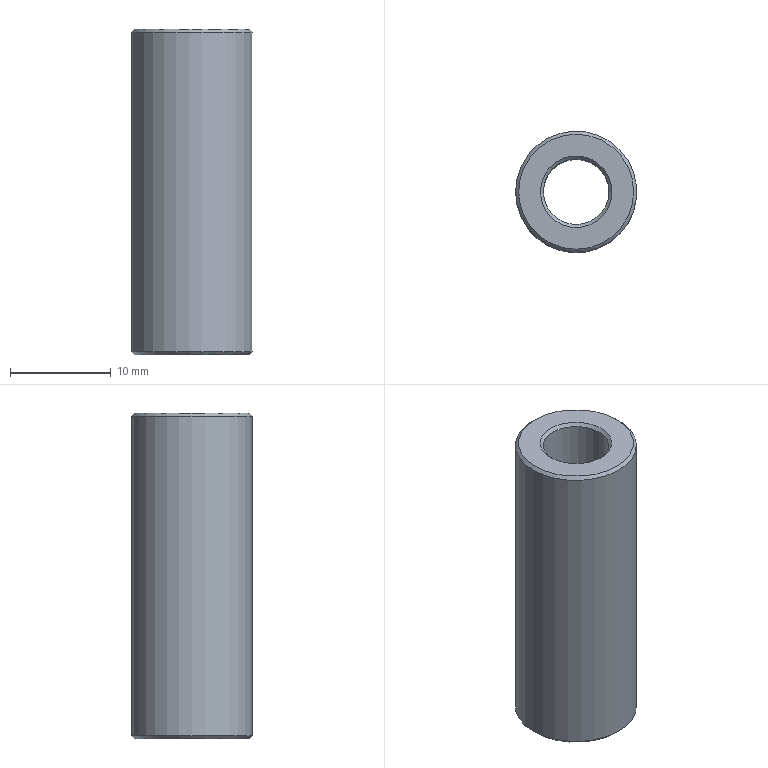Part | STEP file | 200 mesh_id1326 | 1 solid | 8 faces | box 12 x 12 x 32.3 mm | volume 2576 mm3 | cone 4 | plane 2 | cylinder 2 | commonest cylinder face diameters 6.5 x1 12 x1
STEP:
#1=CARTESIAN_POINT('',(-16971.698,-4073.269,32.1));
#2=VERTEX_POINT('',#1);
#3=CARTESIAN_POINT('',(-16968.148,-4073.269,32.1));
#4=DIRECTION('',(0.,0.,-1.));
#5=DIRECTION('',(-1.,0.,0.));
#6=AXIS2_PLACEMENT_3D('',#3,#4,#5);
#7=CIRCLE('',#6,3.55);
#8=EDGE_CURVE('',#2,#2,#7,.T.);
#9=ORIENTED_EDGE('',*,*,#8,.T.);
#10=EDGE_LOOP('',(#9));
#11=FACE_BOUND('',#10,.T.);
#12=CARTESIAN_POINT('',(-16973.848,-4073.269,32.1));
#13=VERTEX_POINT('',#12);
#14=CARTESIAN_POINT('',(-16968.148,-4073.269,32.1));
#15=DIRECTION('',(0.,0.,1.));
#16=DIRECTION('',(-1.,0.,0.));
#17=AXIS2_PLACEMENT_3D('',#14,#15,#16);
#18=CIRCLE('',#17,5.7);
#19=EDGE_CURVE('',#13,#13,#18,.T.);
#20=ORIENTED_EDGE('',*,*,#19,.T.);
#21=EDGE_LOOP('',(#20));
#22=FACE_BOUND('',#21,.T.);
#23=CARTESIAN_POINT('',(-16968.148,-4073.269,32.1));
#24=DIRECTION('',(0.,0.,1.));
#25=DIRECTION('',(-1.,0.,0.));
#26=AXIS2_PLACEMENT_3D('',#23,#24,#25);
#27=PLANE('',#26);
#28=ADVANCED_FACE('',(#11,#22),#27,.T.);
#29=CARTESIAN_POINT('',(-16974.148,-4073.269,0.1));
#30=VERTEX_POINT('',#29);
#31=CARTESIAN_POINT('',(-16968.148,-4073.269,0.1));
#32=DIRECTION('',(0.,0.,1.));
#33=DIRECTION('',(-1.,0.,0.));
#34=AXIS2_PLACEMENT_3D('',#31,#32,#33);
#35=CIRCLE('',#34,6.);
#36=EDGE_CURVE('',#30,#30,#35,.T.);
#37=ORIENTED_EDGE('',*,*,#36,.T.);
#38=EDGE_LOOP('',(#37));
#39=FACE_BOUND('',#38,.T.);
#40=CARTESIAN_POINT('',(-16974.148,-4073.269,31.8));
#41=VERTEX_POINT('',#40);
#42=CARTESIAN_POINT('',(-16968.148,-4073.269,31.8));
#43=DIRECTION('',(0.,0.,-1.));
#44=DIRECTION('',(-1.,0.,0.));
#45=AXIS2_PLACEMENT_3D('',#42,#43,#44);
#46=CIRCLE('',#45,6.);
#47=EDGE_CURVE('',#41,#41,#46,.T.);
#48=ORIENTED_EDGE('',*,*,#47,.T.);
#49=EDGE_LOOP('',(#48));
#50=FACE_BOUND('',#49,.T.);
#51=CARTESIAN_POINT('',(-16968.148,-4073.269,32.4));
#52=DIRECTION('',(0.,0.,-1.));
#53=DIRECTION('',(-1.,0.,0.));
#54=AXIS2_PLACEMENT_3D('',#51,#52,#53);
#55=CYLINDRICAL_SURFACE('',#54,6.);
#56=ADVANCED_FACE('',(#39,#50),#55,.T.);
#57=CARTESIAN_POINT('',(-16971.698,-4073.269,-0.2));
#58=VERTEX_POINT('',#57);
#59=CARTESIAN_POINT('',(-16968.148,-4073.269,-0.2));
#60=DIRECTION('',(0.,0.,1.));
#61=DIRECTION('',(-1.,0.,0.));
#62=AXIS2_PLACEMENT_3D('',#59,#60,#61);
#63=CIRCLE('',#62,3.55);
#64=EDGE_CURVE('',#58,#58,#63,.T.);
#65=ORIENTED_EDGE('',*,*,#64,.T.);
#66=EDGE_LOOP('',(#65));
#67=FACE_BOUND('',#66,.T.);
#68=CARTESIAN_POINT('',(-16973.848,-4073.269,-0.2));
#69=VERTEX_POINT('',#68);
#70=CARTESIAN_POINT('',(-16968.148,-4073.269,-0.2));
#71=DIRECTION('',(0.,0.,-1.));
#72=DIRECTION('',(-1.,0.,0.));
#73=AXIS2_PLACEMENT_3D('',#70,#71,#72);
#74=CIRCLE('',#73,5.7);
#75=EDGE_CURVE('',#69,#69,#74,.T.);
#76=ORIENTED_EDGE('',*,*,#75,.T.);
#77=EDGE_LOOP('',(#76));
#78=FACE_BOUND('',#77,.T.);
#79=CARTESIAN_POINT('',(-16968.148,-4073.269,-0.2));
#80=DIRECTION('',(0.,0.,1.));
#81=DIRECTION('',(-1.,0.,0.));
#82=AXIS2_PLACEMENT_3D('',#79,#80,#81);
#83=PLANE('',#82);
#84=ADVANCED_FACE('',(#67,#78),#83,.F.);
#85=CARTESIAN_POINT('',(-16971.398,-4073.269,0.1));
#86=VERTEX_POINT('',#85);
#87=CARTESIAN_POINT('',(-16968.148,-4073.269,0.1));
#88=DIRECTION('',(0.,0.,-1.));
#89=DIRECTION('',(-1.,0.,0.));
#90=AXIS2_PLACEMENT_3D('',#87,#88,#89);
#91=CIRCLE('',#90,3.25);
#92=EDGE_CURVE('',#86,#86,#91,.T.);
#93=ORIENTED_EDGE('',*,*,#92,.T.);
#94=EDGE_LOOP('',(#93));
#95=FACE_BOUND('',#94,.T.);
#96=CARTESIAN_POINT('',(-16971.398,-4073.269,31.8));
#97=VERTEX_POINT('',#96);
#98=CARTESIAN_POINT('',(-16968.148,-4073.269,31.8));
#99=DIRECTION('',(0.,0.,1.));
#100=DIRECTION('',(-1.,0.,0.));
#101=AXIS2_PLACEMENT_3D('',#98,#99,#100);
#102=CIRCLE('',#101,3.25);
#103=EDGE_CURVE('',#97,#97,#102,.T.);
#104=ORIENTED_EDGE('',*,*,#103,.T.);
#105=EDGE_LOOP('',(#104));
#106=FACE_BOUND('',#105,.T.);
#107=CARTESIAN_POINT('',(-16968.148,-4073.269,32.4));
#108=DIRECTION('',(0.,0.,-1.));
#109=DIRECTION('',(1.,0.,0.));
#110=AXIS2_PLACEMENT_3D('',#107,#108,#109);
#111=CYLINDRICAL_SURFACE('',#110,3.25);
#112=ADVANCED_FACE('',(#95,#106),#111,.F.);
#113=ORIENTED_EDGE('',*,*,#103,.F.);
#114=EDGE_LOOP('',(#113));
#115=FACE_BOUND('',#114,.T.);
#116=ORIENTED_EDGE('',*,*,#8,.F.);
#117=EDGE_LOOP('',(#116));
#118=FACE_BOUND('',#117,.T.);
#119=CARTESIAN_POINT('',(-16968.148,-4073.269,32.1));
#120=DIRECTION('',(0.,0.,1.));
#121=DIRECTION('',(-1.,0.,0.));
#122=AXIS2_PLACEMENT_3D('',#119,#120,#121);
#123=CONICAL_SURFACE('',#122,3.55,45.);
#124=ADVANCED_FACE('',(#115,#118),#123,.F.);
#125=ORIENTED_EDGE('',*,*,#19,.F.);
#126=EDGE_LOOP('',(#125));
#127=FACE_BOUND('',#126,.T.);
#128=ORIENTED_EDGE('',*,*,#47,.F.);
#129=EDGE_LOOP('',(#128));
#130=FACE_BOUND('',#129,.T.);
#131=CARTESIAN_POINT('',(-16968.148,-4073.269,31.8));
#132=DIRECTION('',(0.,0.,-1.));
#133=DIRECTION('',(1.,0.,0.));
#134=AXIS2_PLACEMENT_3D('',#131,#132,#133);
#135=CONICAL_SURFACE('',#134,6.,45.);
#136=ADVANCED_FACE('',(#127,#130),#135,.T.);
#137=ORIENTED_EDGE('',*,*,#92,.F.);
#138=EDGE_LOOP('',(#137));
#139=FACE_BOUND('',#138,.T.);
#140=ORIENTED_EDGE('',*,*,#64,.F.);
#141=EDGE_LOOP('',(#140));
#142=FACE_BOUND('',#141,.T.);
#143=CARTESIAN_POINT('',(-16968.148,-4073.269,-0.2));
#144=DIRECTION('',(0.,0.,-1.));
#145=DIRECTION('',(1.,0.,0.));
#146=AXIS2_PLACEMENT_3D('',#143,#144,#145);
#147=CONICAL_SURFACE('',#146,3.55,45.);
#148=ADVANCED_FACE('',(#139,#142),#147,.F.);
#149=ORIENTED_EDGE('',*,*,#75,.F.);
#150=EDGE_LOOP('',(#149));
#151=FACE_BOUND('',#150,.T.);
#152=ORIENTED_EDGE('',*,*,#36,.F.);
#153=EDGE_LOOP('',(#152));
#154=FACE_BOUND('',#153,.T.);
#155=CARTESIAN_POINT('',(-16968.148,-4073.269,0.1));
#156=DIRECTION('',(0.,0.,1.));
#157=DIRECTION('',(-1.,0.,0.));
#158=AXIS2_PLACEMENT_3D('',#155,#156,#157);
#159=CONICAL_SURFACE('',#158,6.,45.);
#160=ADVANCED_FACE('',(#151,#154),#159,.T.);
#161=CLOSED_SHELL('',(#28,#56,#84,#112,#124,#136,#148,#160));
#162=MANIFOLD_SOLID_BREP('',#161);
#163=(LENGTH_UNIT()NAMED_UNIT(*)SI_UNIT(.MILLI.,.METRE.));
#164=UNCERTAINTY_MEASURE_WITH_UNIT(LENGTH_MEASURE(0.00002),#163,'','');
#165=(NAMED_UNIT(*)PLANE_ANGLE_UNIT()SI_UNIT($,.RADIAN.));
#166=PLANE_ANGLE_MEASURE_WITH_UNIT(PLANE_ANGLE_MEASURE(0.01745),#165);
#167=DIMENSIONAL_EXPONENTS(0.,0.,0.,0.,0.,0.,0.);
#168=(CONVERSION_BASED_UNIT('DEGREE',#166)NAMED_UNIT(#167)PLANE_ANGLE_UNIT());
#169=(NAMED_UNIT(*)SI_UNIT($,.STERADIAN.)SOLID_ANGLE_UNIT());
#170=(GEOMETRIC_REPRESENTATION_CONTEXT(3)GLOBAL_UNCERTAINTY_ASSIGNED_CONTEXT((#164))GLOBAL_UNIT_ASSIGNED_CONTEXT((#163,#168,#169))REPRESENTATION_CONTEXT('',''));
#171=ADVANCED_BREP_SHAPE_REPRESENTATION('',(#162),#170);